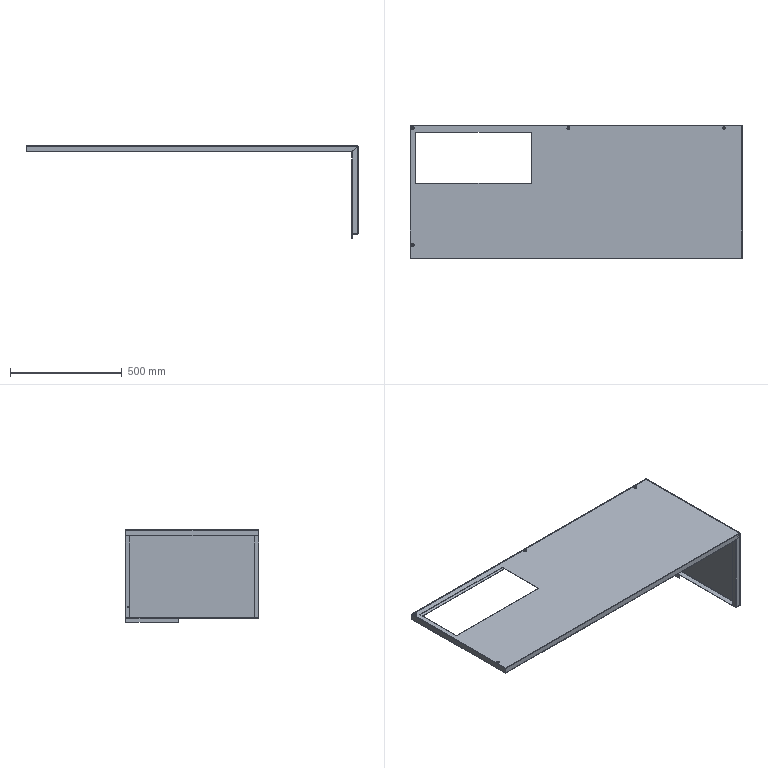Part | STEP file | Right Side Panel | 1 solid | 138 faces | box 1489 x 597 x 416 mm | volume 1815164 mm3 | plane 76 | cylinder 46 | spline 16 | commonest cylinder face diameters 1 x13 4 x13 7 x10 13 x10